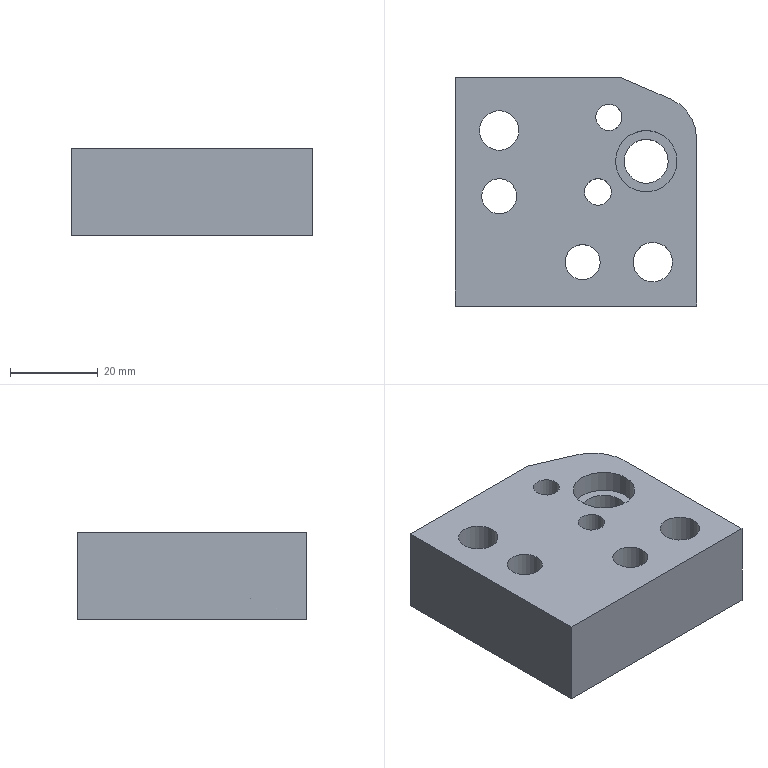Part | STEP file | 413_id2402_x_t | 1 solid | 25 faces | box 55 x 52 x 20 mm | volume 45753 mm3 | cylinder 13 | plane 12 | commonest cylinder face diameters 10 x3 14 x3 8 x2 9 x2 6 x1 6.1 x1